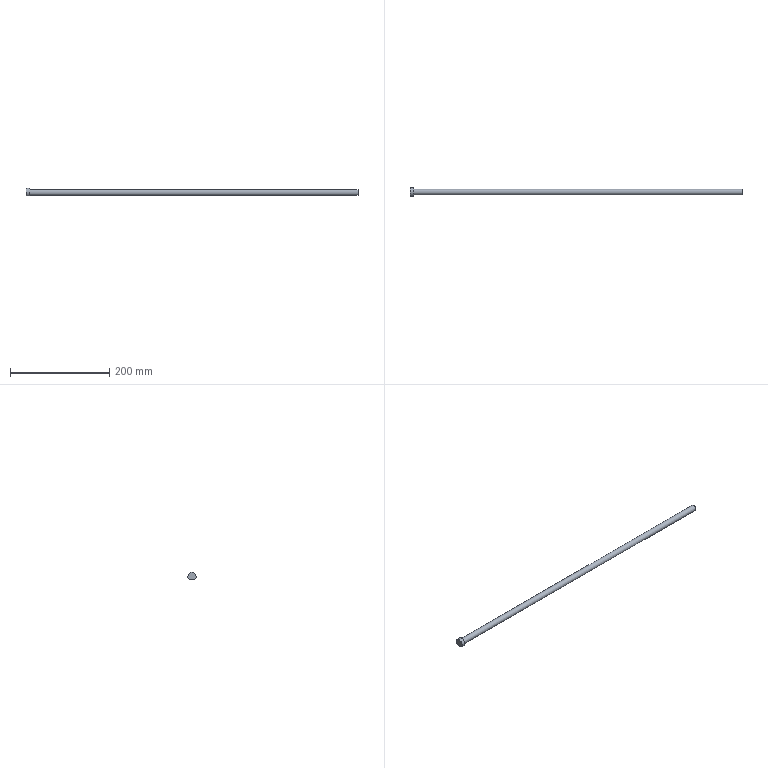Part | STEP file | solid 33 | 1 solid | 6 faces | box 670 x 17 x 15 mm | volume 76566 mm3 | plane 4 | cylinder 2 | commonest cylinder face diameters 12 x1 17 x1